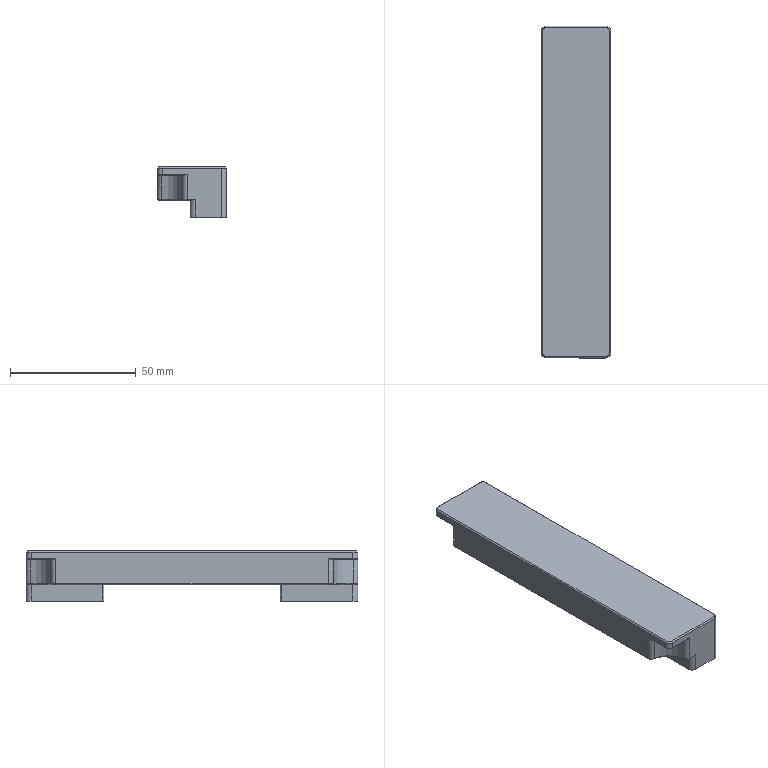NC program | NX | posted with a generic post | part box 27.5 x 132 x 20 mm
Whole program:
N10 G17 G21 G94 G90
(FLOOR_WALL_COPY , TOOL : D80)
N12 T19 M6
N14 G54
N16 G17 G0 G90 X109. Y0. S6500 M3
N18 G43 Z30. H19
N20 Z7.
N22 G94 G1 Z4. F1500.
N24 X106.
N26 X-106.
N28 X-109.
N30 Z7.
N32 G0 Z30.
N34 X109.
N36 Z6.
N38 G1 Z3.
N40 X106.
N42 X-106.
N44 X-109.
N46 Z6.
N48 G0 Z30.
N50 X109.
N52 Z5.
N54 G1 Z2.
N56 X106.
N58 X-106.
N60 X-109.
N62 Z5.
N64 G0 Z30.
N66 X109.
N68 Z4.
N70 G1 Z1.
N72 X106.
N74 X-106.
N76 X-109.
N78 Z4.
N80 G0 Z30.
N82 X109.
N84 Z3.
N86 G1 Z0.
N88 X106.
N90 X-106.
N92 X-109.
N94 Z3.
N96 G0 Z30.
N98 M5
(PLANAR_MILL_COPY_COPY_COPY_COPY_COPY_1 , TOOL : D6A45)
N100 T01 M6
N102 G54
N104 G17 G0 G90 X1.27 Y-15.95 S9500 M3
N106 G43 Z30. H1
N108 Z0.
N110 G94 G1 Z-1.5 F1250.
N112 X0.866 Y-15.25
N114 G3 X0. Y-14.75 R1.
N116 G1 X-64.
N118 G2 X-67. Y-11.75 R3.
N120 G1 Y11.75
N122 G2 X-64. Y14.75 R3.
N124 G1 X64.
N126 G2 X67. Y11.75 R3.
N128 G1 Y-11.75
N130 G2 X64. Y-14.75 R3.
N132 G1 X0.
N134 G3 X-0.866 Y-15.25 R1.
N136 G1 X-1.27 Y-15.95
N138 Z0.
N140 G0 Z30.
N142 M5
N144 M2